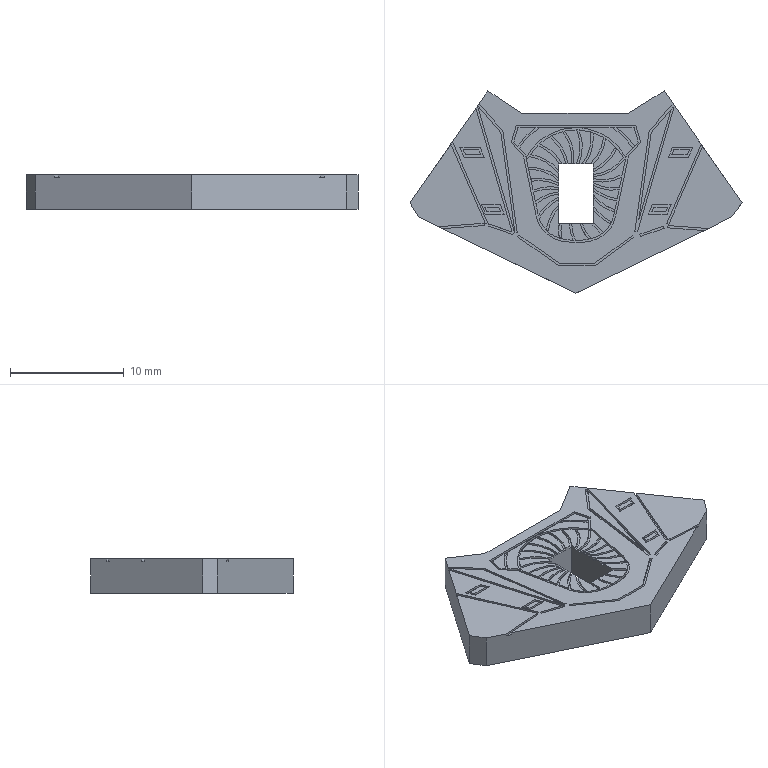Part | SolidWorks | features BaseBody 1 | 1 solid | 260 faces | box 29.201 x 17.776 x 3 mm | volume 913.364 mm3 | plane 181 | spline 79